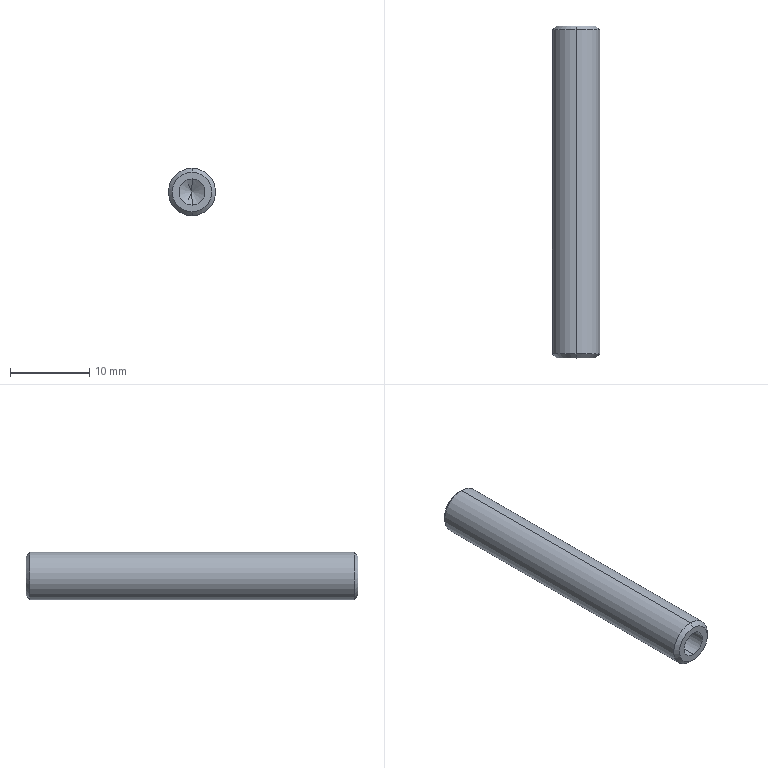Part | STEP file | 0-09-18 Guide shaft D6X50 | 1 solid | 16 faces | box 6 x 42 x 6 mm | volume 1005 mm3 | cone 8 | cylinder 6 | plane 2 | commonest cylinder face diameters 3.3 x4 6 x2
STEP:
#1=CARTESIAN_POINT('',(0.,0.,0.));
#2=DIRECTION('',(0.,0.,1.));
#3=DIRECTION('',(1.,0.,0.));
#4=AXIS2_PLACEMENT_3D('',#1,#2,#3);
#5=CARTESIAN_POINT('',(0.,10.1,-1.65));
#6=VERTEX_POINT('',#5);
#7=CARTESIAN_POINT('',(0.,0.,-1.65));
#8=VERTEX_POINT('',#7);
#9=CARTESIAN_POINT('',(0.,0.,-1.65));
#10=DIRECTION('',(0.,-1.,0.));
#11=VECTOR('',#10,1.);
#12=LINE('',#9,#11);
#13=CARTESIAN_POINT('',(0.,0.,0.));
#14=DIRECTION('',(0.,-1.,0.));
#15=DIRECTION('',(0.,0.,-1.));
#16=AXIS2_PLACEMENT_3D('',#13,#14,#15);
#17=CYLINDRICAL_SURFACE('',#16,1.65);
#18=CARTESIAN_POINT('',(6.283,0.));
#19=DIRECTION('',(0.,1.));
#20=VECTOR('',#19,1.);
#21=LINE('',#18,#20);
#22=(GEOMETRIC_REPRESENTATION_CONTEXT(2)PARAMETRIC_REPRESENTATION_CONTEXT()REPRESENTATION_CONTEXT('',''));
#23=DEFINITIONAL_REPRESENTATION('',(#21),#22);
#24=PCURVE('',#17,#23);
#25=CARTESIAN_POINT('',(0.,0.,0.));
#26=DIRECTION('',(0.,-1.,0.));
#27=DIRECTION('',(0.,0.,-1.));
#28=AXIS2_PLACEMENT_3D('',#25,#26,#27);
#29=CYLINDRICAL_SURFACE('',#28,1.65);
#30=CARTESIAN_POINT('',(0.,0.));
#31=DIRECTION('',(0.,1.));
#32=VECTOR('',#31,1.);
#33=LINE('',#30,#32);
#34=(GEOMETRIC_REPRESENTATION_CONTEXT(2)PARAMETRIC_REPRESENTATION_CONTEXT()REPRESENTATION_CONTEXT('',''));
#35=DEFINITIONAL_REPRESENTATION('',(#33),#34);
#36=PCURVE('',#29,#35);
#37=SURFACE_CURVE('',#12,(#24,#36),.PCURVE_S1.);
#38=EDGE_CURVE('',#6,#8,#37,.T.);
#39=ORIENTED_EDGE('',*,*,#38,.T.);
#40=CARTESIAN_POINT('',(0.,0.,1.65));
#41=VERTEX_POINT('',#40);
#42=CARTESIAN_POINT('',(0.,0.,0.));
#43=DIRECTION('',(0.,-1.,0.));
#44=DIRECTION('',(0.,0.,-1.));
#45=AXIS2_PLACEMENT_3D('',#42,#43,#44);
#46=CIRCLE('',#45,1.65);
#47=CARTESIAN_POINT('',(0.,0.));
#48=DIRECTION('',(1.,0.));
#49=VECTOR('',#48,1.);
#50=LINE('',#47,#49);
#51=(GEOMETRIC_REPRESENTATION_CONTEXT(2)PARAMETRIC_REPRESENTATION_CONTEXT()REPRESENTATION_CONTEXT('',''));
#52=DEFINITIONAL_REPRESENTATION('',(#50),#51);
#53=PCURVE('',#17,#52);
#54=CARTESIAN_POINT('',(0.,0.,0.));
#55=DIRECTION('',(0.,1.,0.));
#56=DIRECTION('',(0.,0.,1.));
#57=AXIS2_PLACEMENT_3D('',#54,#55,#56);
#58=PLANE('',#57);
#59=CARTESIAN_POINT('',(-1.65,0.));
#60=CARTESIAN_POINT('',(-1.65,2.858));
#61=CARTESIAN_POINT('',(0.825,1.429));
#62=CARTESIAN_POINT('',(3.3,0.));
#63=CARTESIAN_POINT('',(0.825,-1.429));
#64=CARTESIAN_POINT('',(-1.65,-2.858));
#65=CARTESIAN_POINT('',(-1.65,0.));
#66=(BOUNDED_CURVE()B_SPLINE_CURVE(2,(#59,#60,#61,#62,#63,#64,#65),.UNSPECIFIED.,.T.,.F.)B_SPLINE_CURVE_WITH_KNOTS((1,2,2,2,2,1),(-2.094,0.,2.094,4.189,6.283,8.378),.UNSPECIFIED.)CURVE()GEOMETRIC_REPRESENTATION_ITEM()RATIONAL_B_SPLINE_CURVE((1.,0.5,1.,0.5,1.,0.5,1.))REPRESENTATION_ITEM(''));
#67=(GEOMETRIC_REPRESENTATION_CONTEXT(2)PARAMETRIC_REPRESENTATION_CONTEXT()REPRESENTATION_CONTEXT('',''));
#68=DEFINITIONAL_REPRESENTATION('',(#66),#67);
#69=PCURVE('',#58,#68);
#70=SURFACE_CURVE('',#46,(#53,#69),.PCURVE_S1.);
#71=EDGE_CURVE('',#41,#8,#70,.T.);
#72=ORIENTED_EDGE('',*,*,#71,.F.);
#73=CARTESIAN_POINT('',(0.,10.1,1.65));
#74=VERTEX_POINT('',#73);
#75=CARTESIAN_POINT('',(0.,0.,1.65));
#76=DIRECTION('',(0.,-1.,0.));
#77=VECTOR('',#76,1.);
#78=LINE('',#75,#77);
#79=CARTESIAN_POINT('',(3.142,0.));
#80=DIRECTION('',(0.,1.));
#81=VECTOR('',#80,1.);
#82=LINE('',#79,#81);
#83=(GEOMETRIC_REPRESENTATION_CONTEXT(2)PARAMETRIC_REPRESENTATION_CONTEXT()REPRESENTATION_CONTEXT('',''));
#84=DEFINITIONAL_REPRESENTATION('',(#82),#83);
#85=PCURVE('',#17,#84);
#86=CARTESIAN_POINT('',(3.142,0.));
#87=DIRECTION('',(0.,1.));
#88=VECTOR('',#87,1.);
#89=LINE('',#86,#88);
#90=(GEOMETRIC_REPRESENTATION_CONTEXT(2)PARAMETRIC_REPRESENTATION_CONTEXT()REPRESENTATION_CONTEXT('',''));
#91=DEFINITIONAL_REPRESENTATION('',(#89),#90);
#92=PCURVE('',#29,#91);
#93=SURFACE_CURVE('',#78,(#85,#92),.PCURVE_S1.);
#94=EDGE_CURVE('',#74,#41,#93,.T.);
#95=ORIENTED_EDGE('',*,*,#94,.F.);
#96=CARTESIAN_POINT('',(0.,10.1,0.));
#97=DIRECTION('',(0.,-1.,0.));
#98=DIRECTION('',(0.,0.,-1.));
#99=AXIS2_PLACEMENT_3D('',#96,#97,#98);
#100=CIRCLE('',#99,1.65);
#101=CARTESIAN_POINT('',(0.,-10.1));
#102=DIRECTION('',(1.,0.));
#103=VECTOR('',#102,1.);
#104=LINE('',#101,#103);
#105=(GEOMETRIC_REPRESENTATION_CONTEXT(2)PARAMETRIC_REPRESENTATION_CONTEXT()REPRESENTATION_CONTEXT('',''));
#106=DEFINITIONAL_REPRESENTATION('',(#104),#105);
#107=PCURVE('',#17,#106);
#108=CARTESIAN_POINT('',(0.,10.1,0.));
#109=DIRECTION('',(0.,-1.,0.));
#110=DIRECTION('',(0.,0.,-1.));
#111=AXIS2_PLACEMENT_3D('',#108,#109,#110);
#112=CONICAL_SURFACE('',#111,1.65,1.03);
#113=CARTESIAN_POINT('',(0.,0.));
#114=DIRECTION('',(1.,0.));
#115=VECTOR('',#114,1.);
#116=LINE('',#113,#115);
#117=(GEOMETRIC_REPRESENTATION_CONTEXT(2)PARAMETRIC_REPRESENTATION_CONTEXT()REPRESENTATION_CONTEXT('',''));
#118=DEFINITIONAL_REPRESENTATION('',(#116),#117);
#119=PCURVE('',#112,#118);
#120=SURFACE_CURVE('',#100,(#107,#119),.PCURVE_S1.);
#121=EDGE_CURVE('',#74,#6,#120,.T.);
#122=ORIENTED_EDGE('',*,*,#121,.T.);
#123=EDGE_LOOP('',(#39,#72,#95,#122));
#124=FACE_BOUND('',#123,.F.);
#125=ADVANCED_FACE('',(#124),#17,.F.);
#126=ORIENTED_EDGE('',*,*,#121,.F.);
#127=CARTESIAN_POINT('',(0.,11.091,0.));
#128=VERTEX_POINT('',#127);
#129=CARTESIAN_POINT('',(0.,10.1,1.65));
#130=DIRECTION('',(0.,-0.515,0.8572));
#131=VECTOR('',#130,1.);
#132=LINE('',#129,#131);
#133=CARTESIAN_POINT('',(3.142,0.));
#134=DIRECTION('',(0.,1.));
#135=VECTOR('',#134,1.);
#136=LINE('',#133,#135);
#137=(GEOMETRIC_REPRESENTATION_CONTEXT(2)PARAMETRIC_REPRESENTATION_CONTEXT()REPRESENTATION_CONTEXT('',''));
#138=DEFINITIONAL_REPRESENTATION('',(#136),#137);
#139=PCURVE('',#112,#138);
#140=CARTESIAN_POINT('',(0.,10.1,0.));
#141=DIRECTION('',(0.,-1.,0.));
#142=DIRECTION('',(0.,0.,-1.));
#143=AXIS2_PLACEMENT_3D('',#140,#141,#142);
#144=CONICAL_SURFACE('',#143,1.65,1.03);
#145=CARTESIAN_POINT('',(3.142,0.));
#146=DIRECTION('',(0.,1.));
#147=VECTOR('',#146,1.);
#148=LINE('',#145,#147);
#149=(GEOMETRIC_REPRESENTATION_CONTEXT(2)PARAMETRIC_REPRESENTATION_CONTEXT()REPRESENTATION_CONTEXT('',''));
#150=DEFINITIONAL_REPRESENTATION('',(#148),#149);
#151=PCURVE('',#144,#150);
#152=SURFACE_CURVE('',#132,(#139,#151),.PCURVE_S1.);
#153=EDGE_CURVE('',#128,#74,#152,.T.);
#154=ORIENTED_EDGE('',*,*,#153,.F.);
#155=CARTESIAN_POINT('',(0.,10.1,-1.65));
#156=DIRECTION('',(0.,-0.515,-0.8572));
#157=VECTOR('',#156,1.);
#158=LINE('',#155,#157);
#159=CARTESIAN_POINT('',(6.283,0.));
#160=DIRECTION('',(0.,1.));
#161=VECTOR('',#160,1.);
#162=LINE('',#159,#161);
#163=(GEOMETRIC_REPRESENTATION_CONTEXT(2)PARAMETRIC_REPRESENTATION_CONTEXT()REPRESENTATION_CONTEXT('',''));
#164=DEFINITIONAL_REPRESENTATION('',(#162),#163);
#165=PCURVE('',#112,#164);
#166=CARTESIAN_POINT('',(0.,0.));
#167=DIRECTION('',(0.,1.));
#168=VECTOR('',#167,1.);
#169=LINE('',#166,#168);
#170=(GEOMETRIC_REPRESENTATION_CONTEXT(2)PARAMETRIC_REPRESENTATION_CONTEXT()REPRESENTATION_CONTEXT('',''));
#171=DEFINITIONAL_REPRESENTATION('',(#169),#170);
#172=PCURVE('',#144,#171);
#173=SURFACE_CURVE('',#158,(#165,#172),.PCURVE_S1.);
#174=EDGE_CURVE('',#128,#6,#173,.T.);
#175=ORIENTED_EDGE('',*,*,#174,.T.);
#176=EDGE_LOOP('',(#126,#154,#175));
#177=FACE_BOUND('',#176,.F.);
#178=ADVANCED_FACE('',(#177),#112,.F.);
#179=CARTESIAN_POINT('',(0.,31.9,1.65));
#180=VERTEX_POINT('',#179);
#181=CARTESIAN_POINT('',(0.,42.,1.65));
#182=VERTEX_POINT('',#181);
#183=CARTESIAN_POINT('',(0.,42.,1.65));
#184=DIRECTION('',(0.,1.,0.));
#185=VECTOR('',#184,1.);
#186=LINE('',#183,#185);
#187=CARTESIAN_POINT('',(0.,42.,0.));
#188=DIRECTION('',(0.,1.,0.));
#189=DIRECTION('',(0.,0.,1.));
#190=AXIS2_PLACEMENT_3D('',#187,#188,#189);
#191=CYLINDRICAL_SURFACE('',#190,1.65);
#192=CARTESIAN_POINT('',(6.283,0.));
#193=DIRECTION('',(0.,1.));
#194=VECTOR('',#193,1.);
#195=LINE('',#192,#194);
#196=(GEOMETRIC_REPRESENTATION_CONTEXT(2)PARAMETRIC_REPRESENTATION_CONTEXT()REPRESENTATION_CONTEXT('',''));
#197=DEFINITIONAL_REPRESENTATION('',(#195),#196);
#198=PCURVE('',#191,#197);
#199=CARTESIAN_POINT('',(0.,42.,0.));
#200=DIRECTION('',(0.,1.,0.));
#201=DIRECTION('',(0.,0.,1.));
#202=AXIS2_PLACEMENT_3D('',#199,#200,#201);
#203=CYLINDRICAL_SURFACE('',#202,1.65);
#204=CARTESIAN_POINT('',(0.,0.));
#205=DIRECTION('',(0.,1.));
#206=VECTOR('',#205,1.);
#207=LINE('',#204,#206);
#208=(GEOMETRIC_REPRESENTATION_CONTEXT(2)PARAMETRIC_REPRESENTATION_CONTEXT()REPRESENTATION_CONTEXT('',''));
#209=DEFINITIONAL_REPRESENTATION('',(#207),#208);
#210=PCURVE('',#203,#209);
#211=SURFACE_CURVE('',#186,(#198,#210),.PCURVE_S1.);
#212=EDGE_CURVE('',#180,#182,#211,.T.);
#213=ORIENTED_EDGE('',*,*,#212,.T.);
#214=CARTESIAN_POINT('',(0.,42.,-1.65));
#215=VERTEX_POINT('',#214);
#216=CARTESIAN_POINT('',(0.,42.,0.));
#217=DIRECTION('',(0.,1.,0.));
#218=DIRECTION('',(0.,0.,1.));
#219=AXIS2_PLACEMENT_3D('',#216,#217,#218);
#220=CIRCLE('',#219,1.65);
#221=CARTESIAN_POINT('',(0.,0.));
#222=DIRECTION('',(1.,0.));
#223=VECTOR('',#222,1.);
#224=LINE('',#221,#223);
#225=(GEOMETRIC_REPRESENTATION_CONTEXT(2)PARAMETRIC_REPRESENTATION_CONTEXT()REPRESENTATION_CONTEXT('',''));
#226=DEFINITIONAL_REPRESENTATION('',(#224),#225);
#227=PCURVE('',#191,#226);
#228=CARTESIAN_POINT('',(0.,42.,0.));
#229=DIRECTION('',(0.,-1.,0.));
#230=DIRECTION('',(0.,0.,-1.));
#231=AXIS2_PLACEMENT_3D('',#228,#229,#230);
#232=PLANE('',#231);
#233=CARTESIAN_POINT('',(-1.65,0.));
#234=CARTESIAN_POINT('',(-1.65,2.858));
#235=CARTESIAN_POINT('',(0.825,1.429));
#236=CARTESIAN_POINT('',(3.3,0.));
#237=CARTESIAN_POINT('',(0.825,-1.429));
#238=CARTESIAN_POINT('',(-1.65,-2.858));
#239=CARTESIAN_POINT('',(-1.65,0.));
#240=(BOUNDED_CURVE()B_SPLINE_CURVE(2,(#233,#234,#235,#236,#237,#238,#239),.UNSPECIFIED.,.T.,.F.)B_SPLINE_CURVE_WITH_KNOTS((1,2,2,2,2,1),(-2.094,0.,2.094,4.189,6.283,8.378),.UNSPECIFIED.)CURVE()GEOMETRIC_REPRESENTATION_ITEM()RATIONAL_B_SPLINE_CURVE((1.,0.5,1.,0.5,1.,0.5,1.))REPRESENTATION_ITEM(''));
#241=(GEOMETRIC_REPRESENTATION_CONTEXT(2)PARAMETRIC_REPRESENTATION_CONTEXT()REPRESENTATION_CONTEXT('',''));
#242=DEFINITIONAL_REPRESENTATION('',(#240),#241);
#243=PCURVE('',#232,#242);
#244=SURFACE_CURVE('',#220,(#227,#243),.PCURVE_S1.);
#245=EDGE_CURVE('',#215,#182,#244,.T.);
#246=ORIENTED_EDGE('',*,*,#245,.F.);
#247=CARTESIAN_POINT('',(0.,31.9,-1.65));
#248=VERTEX_POINT('',#247);
#249=CARTESIAN_POINT('',(0.,42.,-1.65));
#250=DIRECTION('',(0.,1.,0.));
#251=VECTOR('',#250,1.);
#252=LINE('',#249,#251);
#253=CARTESIAN_POINT('',(3.142,0.));
#254=DIRECTION('',(0.,1.));
#255=VECTOR('',#254,1.);
#256=LINE('',#253,#255);
#257=(GEOMETRIC_REPRESENTATION_CONTEXT(2)PARAMETRIC_REPRESENTATION_CONTEXT()REPRESENTATION_CONTEXT('',''));
#258=DEFINITIONAL_REPRESENTATION('',(#256),#257);
#259=PCURVE('',#191,#258);
#260=CARTESIAN_POINT('',(3.142,0.));
#261=DIRECTION('',(0.,1.));
#262=VECTOR('',#261,1.);
#263=LINE('',#260,#262);
#264=(GEOMETRIC_REPRESENTATION_CONTEXT(2)PARAMETRIC_REPRESENTATION_CONTEXT()REPRESENTATION_CONTEXT('',''));
#265=DEFINITIONAL_REPRESENTATION('',(#263),#264);
#266=PCURVE('',#203,#265);
#267=SURFACE_CURVE('',#252,(#259,#266),.PCURVE_S1.);
#268=EDGE_CURVE('',#248,#215,#267,.T.);
#269=ORIENTED_EDGE('',*,*,#268,.F.);
#270=CARTESIAN_POINT('',(0.,31.9,0.));
#271=DIRECTION('',(0.,1.,0.));
#272=DIRECTION('',(0.,0.,1.));
#273=AXIS2_PLACEMENT_3D('',#270,#271,#272);
#274=CIRCLE('',#273,1.65);
#275=CARTESIAN_POINT('',(0.,-10.1));
#276=DIRECTION('',(1.,0.));
#277=VECTOR('',#276,1.);
#278=LINE('',#275,#277);
#279=(GEOMETRIC_REPRESENTATION_CONTEXT(2)PARAMETRIC_REPRESENTATION_CONTEXT()REPRESENTATION_CONTEXT('',''));
#280=DEFINITIONAL_REPRESENTATION('',(#278),#279);
#281=PCURVE('',#191,#280);
#282=CARTESIAN_POINT('',(0.,31.9,0.));
#283=DIRECTION('',(0.,1.,0.));
#284=DIRECTION('',(0.,0.,1.));
#285=AXIS2_PLACEMENT_3D('',#282,#283,#284);
#286=CONICAL_SURFACE('',#285,1.65,1.03);
#287=CARTESIAN_POINT('',(0.,0.));
#288=DIRECTION('',(1.,0.));
#289=VECTOR('',#288,1.);
#290=LINE('',#287,#289);
#291=(GEOMETRIC_REPRESENTATION_CONTEXT(2)PARAMETRIC_REPRESENTATION_CONTEXT()REPRESENTATION_CONTEXT('',''));
#292=DEFINITIONAL_REPRESENTATION('',(#290),#291);
#293=PCURVE('',#286,#292);
#294=SURFACE_CURVE('',#274,(#281,#293),.PCURVE_S1.);
#295=EDGE_CURVE('',#248,#180,#294,.T.);
#296=ORIENTED_EDGE('',*,*,#295,.T.);
#297=EDGE_LOOP('',(#213,#246,#269,#296));
#298=FACE_BOUND('',#297,.F.);
#299=ADVANCED_FACE('',(#298),#191,.F.);
#300=ORIENTED_EDGE('',*,*,#295,.F.);
#301=CARTESIAN_POINT('',(0.,30.909,0.));
#302=VERTEX_POINT('',#301);
#303=CARTESIAN_POINT('',(0.,31.9,-1.65));
#304=DIRECTION('',(0.,0.515,-0.8572));
#305=VECTOR('',#304,1.);
#306=LINE('',#303,#305);
#307=CARTESIAN_POINT('',(3.142,0.));
#308=DIRECTION('',(0.,1.));
#309=VECTOR('',#308,1.);
#310=LINE('',#307,#309);
#311=(GEOMETRIC_REPRESENTATION_CONTEXT(2)PARAMETRIC_REPRESENTATION_CONTEXT()REPRESENTATION_CONTEXT('',''));
#312=DEFINITIONAL_REPRESENTATION('',(#310),#311);
#313=PCURVE('',#286,#312);
#314=CARTESIAN_POINT('',(0.,31.9,0.));
#315=DIRECTION('',(0.,1.,0.));
#316=DIRECTION('',(0.,0.,1.));
#317=AXIS2_PLACEMENT_3D('',#314,#315,#316);
#318=CONICAL_SURFACE('',#317,1.65,1.03);
#319=CARTESIAN_POINT('',(3.142,0.));
#320=DIRECTION('',(0.,1.));
#321=VECTOR('',#320,1.);
#322=LINE('',#319,#321);
#323=(GEOMETRIC_REPRESENTATION_CONTEXT(2)PARAMETRIC_REPRESENTATION_CONTEXT()REPRESENTATION_CONTEXT('',''));
#324=DEFINITIONAL_REPRESENTATION('',(#322),#323);
#325=PCURVE('',#318,#324);
#326=SURFACE_CURVE('',#306,(#313,#325),.PCURVE_S1.);
#327=EDGE_CURVE('',#302,#248,#326,.T.);
#328=ORIENTED_EDGE('',*,*,#327,.F.);
#329=CARTESIAN_POINT('',(0.,31.9,1.65));
#330=DIRECTION('',(0.,0.515,0.8572));
#331=VECTOR('',#330,1.);
#332=LINE('',#329,#331);
#333=CARTESIAN_POINT('',(6.283,0.));
#334=DIRECTION('',(0.,1.));
#335=VECTOR('',#334,1.);
#336=LINE('',#333,#335);
#337=(GEOMETRIC_REPRESENTATION_CONTEXT(2)PARAMETRIC_REPRESENTATION_CONTEXT()REPRESENTATION_CONTEXT('',''));
#338=DEFINITIONAL_REPRESENTATION('',(#336),#337);
#339=PCURVE('',#286,#338);
#340=CARTESIAN_POINT('',(0.,0.));
#341=DIRECTION('',(0.,1.));
#342=VECTOR('',#341,1.);
#343=LINE('',#340,#342);
#344=(GEOMETRIC_REPRESENTATION_CONTEXT(2)PARAMETRIC_REPRESENTATION_CONTEXT()REPRESENTATION_CONTEXT('',''));
#345=DEFINITIONAL_REPRESENTATION('',(#343),#344);
#346=PCURVE('',#318,#345);
#347=SURFACE_CURVE('',#332,(#339,#346),.PCURVE_S1.);
#348=EDGE_CURVE('',#302,#180,#347,.T.);
#349=ORIENTED_EDGE('',*,*,#348,.T.);
#350=EDGE_LOOP('',(#300,#328,#349));
#351=FACE_BOUND('',#350,.F.);
#352=ADVANCED_FACE('',(#351),#286,.F.);
#353=CARTESIAN_POINT('',(0.,42.,2.5));
#354=VERTEX_POINT('',#353);
#355=CARTESIAN_POINT('',(0.,42.,-2.5));
#356=VERTEX_POINT('',#355);
#357=CARTESIAN_POINT('',(0.,42.,0.));
#358=DIRECTION('',(0.,1.,0.));
#359=DIRECTION('',(0.,0.,-1.));
#360=AXIS2_PLACEMENT_3D('',#357,#358,#359);
#361=CIRCLE('',#360,2.5);
#362=CARTESIAN_POINT('',(0.,41.5,0.));
#363=DIRECTION('',(0.,-1.,0.));
#364=DIRECTION('',(0.,0.,-1.));
#365=AXIS2_PLACEMENT_3D('',#362,#363,#364);
#366=CONICAL_SURFACE('',#365,3.,0.7854);
#367=CARTESIAN_POINT('',(6.283,-0.5));
#368=DIRECTION('',(-1.,0.));
#369=VECTOR('',#368,1.);
#370=LINE('',#367,#369);
#371=(GEOMETRIC_REPRESENTATION_CONTEXT(2)PARAMETRIC_REPRESENTATION_CONTEXT()REPRESENTATION_CONTEXT('',''));
#372=DEFINITIONAL_REPRESENTATION('',(#370),#371);
#373=PCURVE('',#366,#372);
#374=CARTESIAN_POINT('',(2.5,0.));
#375=CARTESIAN_POINT('',(2.5,-4.33));
#376=CARTESIAN_POINT('',(-1.25,-2.165));
#377=CARTESIAN_POINT('',(-5.,0.));
#378=CARTESIAN_POINT('',(-1.25,2.165));
#379=CARTESIAN_POINT('',(2.5,4.33));
#380=CARTESIAN_POINT('',(2.5,0.));
#381=(BOUNDED_CURVE()B_SPLINE_CURVE(2,(#374,#375,#376,#377,#378,#379,#380),.UNSPECIFIED.,.T.,.F.)B_SPLINE_CURVE_WITH_KNOTS((1,2,2,2,2,1),(-2.094,0.,2.094,4.189,6.283,8.378),.UNSPECIFIED.)CURVE()GEOMETRIC_REPRESENTATION_ITEM()RATIONAL_B_SPLINE_CURVE((1.,0.5,1.,0.5,1.,0.5,1.))REPRESENTATION_ITEM(''));
#382=(GEOMETRIC_REPRESENTATION_CONTEXT(2)PARAMETRIC_REPRESENTATION_CONTEXT()REPRESENTATION_CONTEXT('',''));
#383=DEFINITIONAL_REPRESENTATION('',(#381),#382);
#384=PCURVE('',#232,#383);
#385=SURFACE_CURVE('',#361,(#373,#384),.PCURVE_S1.);
#386=EDGE_CURVE('',#354,#356,#385,.T.);
#387=ORIENTED_EDGE('',*,*,#386,.F.);
#388=CARTESIAN_POINT('',(0.,41.5,3.));
#389=VERTEX_POINT('',#388);
#390=CARTESIAN_POINT('',(0.,41.5,3.));
#391=DIRECTION('',(0.,-0.7071,0.7071));
#392=VECTOR('',#391,1.);
#393=LINE('',#390,#392);
#394=CARTESIAN_POINT('',(3.142,0.));
#395=DIRECTION('',(0.,1.));
#396=VECTOR('',#395,1.);
#397=LINE('',#394,#396);
#398=(GEOMETRIC_REPRESENTATION_CONTEXT(2)PARAMETRIC_REPRESENTATION_CONTEXT()REPRESENTATION_CONTEXT('',''));
#399=DEFINITIONAL_REPRESENTATION('',(#397),#398);
#400=PCURVE('',#366,#399);
#401=CARTESIAN_POINT('',(0.,41.5,0.));
#402=DIRECTION('',(0.,-1.,0.));
#403=DIRECTION('',(0.,0.,-1.));
#404=AXIS2_PLACEMENT_3D('',#401,#402,#403);
#405=CONICAL_SURFACE('',#404,3.,0.7854);
#406=CARTESIAN_POINT('',(3.142,0.));
#407=DIRECTION('',(0.,1.));
#408=VECTOR('',#407,1.);
#409=LINE('',#406,#408);
#410=(GEOMETRIC_REPRESENTATION_CONTEXT(2)PARAMETRIC_REPRESENTATION_CONTEXT()REPRESENTATION_CONTEXT('',''));
#411=DEFINITIONAL_REPRESENTATION('',(#409),#410);
#412=PCURVE('',#405,#411);
#413=SURFACE_CURVE('',#393,(#400,#412),.PCURVE_S1.);
#414=EDGE_CURVE('',#354,#389,#413,.T.);
#415=ORIENTED_EDGE('',*,*,#414,.T.);
#416=CARTESIAN_POINT('',(0.,41.5,-3.));
#417=VERTEX_POINT('',#416);
#418=CARTESIAN_POINT('',(0.,41.5,0.));
#419=DIRECTION('',(0.,-1.,0.));
#420=DIRECTION('',(0.,0.,-1.));
#421=AXIS2_PLACEMENT_3D('',#418,#419,#420);
#422=CIRCLE('',#421,3.);
#423=CARTESIAN_POINT('',(0.,0.));
#424=DIRECTION('',(1.,0.));
#425=VECTOR('',#424,1.);
#426=LINE('',#423,#425);
#427=(GEOMETRIC_REPRESENTATION_CONTEXT(2)PARAMETRIC_REPRESENTATION_CONTEXT()REPRESENTATION_CONTEXT('',''));
#428=DEFINITIONAL_REPRESENTATION('',(#426),#427);
#429=PCURVE('',#366,#428);
#430=CARTESIAN_POINT('',(0.,0.,0.));
#431=DIRECTION('',(0.,-1.,0.));
#432=DIRECTION('',(0.,0.,-1.));
#433=AXIS2_PLACEMENT_3D('',#430,#431,#432);
#434=CYLINDRICAL_SURFACE('',#433,3.);
#435=CARTESIAN_POINT('',(0.,-41.5));
#436=DIRECTION('',(1.,0.));
#437=VECTOR('',#436,1.);
#438=LINE('',#435,#437);
#439=(GEOMETRIC_REPRESENTATION_CONTEXT(2)PARAMETRIC_REPRESENTATION_CONTEXT()REPRESENTATION_CONTEXT('',''));
#440=DEFINITIONAL_REPRESENTATION('',(#438),#439);
#441=PCURVE('',#434,#440);
#442=SURFACE_CURVE('',#422,(#429,#441),.PCURVE_S1.);
#443=EDGE_CURVE('',#417,#389,#442,.T.);
#444=ORIENTED_EDGE('',*,*,#443,.F.);
#445=CARTESIAN_POINT('',(0.,41.5,-3.));
#446=DIRECTION('',(0.,-0.7071,-0.7071));
#447=VECTOR('',#446,1.);
#448=LINE('',#445,#447);
#449=CARTESIAN_POINT('',(0.,0.));
#450=DIRECTION('',(0.,1.));
#451=VECTOR('',#450,1.);
#452=LINE('',#449,#451);
#453=(GEOMETRIC_REPRESENTATION_CONTEXT(2)PARAMETRIC_REPRESENTATION_CONTEXT()REPRESENTATION_CONTEXT('',''));
#454=DEFINITIONAL_REPRESENTATION('',(#452),#453);
#455=PCURVE('',#366,#454);
#456=CARTESIAN_POINT('',(6.283,0.));
#457=DIRECTION('',(0.,1.));
#458=VECTOR('',#457,1.);
#459=LINE('',#456,#458);
#460=(GEOMETRIC_REPRESENTATION_CONTEXT(2)PARAMETRIC_REPRESENTATION_CONTEXT()REPRESENTATION_CONTEXT('',''));
#461=DEFINITIONAL_REPRESENTATION('',(#459),#460);
#462=PCURVE('',#405,#461);
#463=SURFACE_CURVE('',#448,(#455,#462),.PCURVE_S1.);
#464=EDGE_CURVE('',#356,#417,#463,.T.);
#465=ORIENTED_EDGE('',*,*,#464,.F.);
#466=EDGE_LOOP('',(#387,#415,#444,#465));
#467=FACE_BOUND('',#466,.T.);
#468=ADVANCED_FACE('',(#467),#366,.T.);
#469=CARTESIAN_POINT('',(0.,0.,-2.5));
#470=VERTEX_POINT('',#469);
#471=CARTESIAN_POINT('',(0.,0.,2.5));
#472=VERTEX_POINT('',#471);
#473=CARTESIAN_POINT('',(0.,0.,0.));
#474=DIRECTION('',(0.,-1.,0.));
#475=DIRECTION('',(0.,0.,1.));
#476=AXIS2_PLACEMENT_3D('',#473,#474,#475);
#477=CIRCLE('',#476,2.5);
#478=CARTESIAN_POINT('',(0.,0.,0.));
#479=DIRECTION('',(0.,1.,0.));
#480=DIRECTION('',(0.,0.,1.));
#481=AXIS2_PLACEMENT_3D('',#478,#479,#480);
#482=CONICAL_SURFACE('',#481,2.5,0.7854);
#483=CARTESIAN_POINT('',(6.283,0.));
#484=DIRECTION('',(-1.,0.));
#485=VECTOR('',#484,1.);
#486=LINE('',#483,#485);
#487=(GEOMETRIC_REPRESENTATION_CONTEXT(2)PARAMETRIC_REPRESENTATION_CONTEXT()REPRESENTATION_CONTEXT('',''));
#488=DEFINITIONAL_REPRESENTATION('',(#486),#487);
#489=PCURVE('',#482,#488);
#490=CARTESIAN_POINT('',(2.5,0.));
#491=CARTESIAN_POINT('',(2.5,-4.33));
#492=CARTESIAN_POINT('',(-1.25,-2.165));
#493=CARTESIAN_POINT('',(-5.,0.));
#494=CARTESIAN_POINT('',(-1.25,2.165));
#495=CARTESIAN_POINT('',(2.5,4.33));
#496=CARTESIAN_POINT('',(2.5,0.));
#497=(BOUNDED_CURVE()B_SPLINE_CURVE(2,(#490,#491,#492,#493,#494,#495,#496),.UNSPECIFIED.,.T.,.F.)B_SPLINE_CURVE_WITH_KNOTS((1,2,2,2,2,1),(-2.094,0.,2.094,4.189,6.283,8.378),.UNSPECIFIED.)CURVE()GEOMETRIC_REPRESENTATION_ITEM()RATIONAL_B_SPLINE_CURVE((1.,0.5,1.,0.5,1.,0.5,1.))REPRESENTATION_ITEM(''));
#498=(GEOMETRIC_REPRESENTATION_CONTEXT(2)PARAMETRIC_REPRESENTATION_CONTEXT()REPRESENTATION_CONTEXT('',''));
#499=DEFINITIONAL_REPRESENTATION('',(#497),#498);
#500=PCURVE('',#58,#499);
#501=SURFACE_CURVE('',#477,(#489,#500),.PCURVE_S1.);
#502=EDGE_CURVE('',#470,#472,#501,.T.);
#503=ORIENTED_EDGE('',*,*,#502,.F.);
#504=CARTESIAN_POINT('',(0.,0.5,-3.));
#505=VERTEX_POINT('',#504);
#506=CARTESIAN_POINT('',(0.,0.,-2.5));
#507=DIRECTION('',(0.,0.7071,-0.7071));
#508=VECTOR('',#507,1.);
#509=LINE('',#506,#508);
#510=CARTESIAN_POINT('',(3.142,0.));
#511=DIRECTION('',(0.,1.));
#512=VECTOR('',#511,1.);
#513=LINE('',#510,#512);
#514=(GEOMETRIC_REPRESENTATION_CONTEXT(2)PARAMETRIC_REPRESENTATION_CONTEXT()REPRESENTATION_CONTEXT('',''));
#515=DEFINITIONAL_REPRESENTATION('',(#513),#514);
#516=PCURVE('',#482,#515);
#517=CARTESIAN_POINT('',(0.,0.,0.));
#518=DIRECTION('',(0.,1.,0.));
#519=DIRECTION('',(0.,0.,1.));
#520=AXIS2_PLACEMENT_3D('',#517,#518,#519);
#521=CONICAL_SURFACE('',#520,2.5,0.7854);
#522=CARTESIAN_POINT('',(3.142,0.));
#523=DIRECTION('',(0.,1.));
#524=VECTOR('',#523,1.);
#525=LINE('',#522,#524);
#526=(GEOMETRIC_REPRESENTATION_CONTEXT(2)PARAMETRIC_REPRESENTATION_CONTEXT()REPRESENTATION_CONTEXT('',''));
#527=DEFINITIONAL_REPRESENTATION('',(#525),#526);
#528=PCURVE('',#521,#527);
#529=SURFACE_CURVE('',#509,(#516,#528),.PCURVE_S1.);
#530=EDGE_CURVE('',#470,#505,#529,.T.);
#531=ORIENTED_EDGE('',*,*,#530,.T.);
#532=CARTESIAN_POINT('',(0.,0.5,3.));
#533=VERTEX_POINT('',#532);
#534=CARTESIAN_POINT('',(0.,0.5,0.));
#535=DIRECTION('',(0.,1.,0.));
#536=DIRECTION('',(0.,0.,1.));
#537=AXIS2_PLACEMENT_3D('',#534,#535,#536);
#538=CIRCLE('',#537,3.);
#539=CARTESIAN_POINT('',(0.,0.5));
#540=DIRECTION('',(1.,0.));
#541=VECTOR('',#540,1.);
#542=LINE('',#539,#541);
#543=(GEOMETRIC_REPRESENTATION_CONTEXT(2)PARAMETRIC_REPRESENTATION_CONTEXT()REPRESENTATION_CONTEXT('',''));
#544=DEFINITIONAL_REPRESENTATION('',(#542),#543);
#545=PCURVE('',#482,#544);
#546=CARTESIAN_POINT('',(3.142,-0.5));
#547=DIRECTION('',(-1.,0.));
#548=VECTOR('',#547,1.);
#549=LINE('',#546,#548);
#550=(GEOMETRIC_REPRESENTATION_CONTEXT(2)PARAMETRIC_REPRESENTATION_CONTEXT()REPRESENTATION_CONTEXT('',''));
#551=DEFINITIONAL_REPRESENTATION('',(#549),#550);
#552=PCURVE('',#434,#551);
#553=SURFACE_CURVE('',#538,(#545,#552),.PCURVE_S1.);
#554=EDGE_CURVE('',#533,#505,#553,.T.);
#555=ORIENTED_EDGE('',*,*,#554,.F.);
#556=CARTESIAN_POINT('',(0.,0.,2.5));
#557=DIRECTION('',(0.,0.7071,0.7071));
#558=VECTOR('',#557,1.);
#559=LINE('',#556,#558);
#560=CARTESIAN_POINT('',(0.,0.));
#561=DIRECTION('',(0.,1.));
#562=VECTOR('',#561,1.);
#563=LINE('',#560,#562);
#564=(GEOMETRIC_REPRESENTATION_CONTEXT(2)PARAMETRIC_REPRESENTATION_CONTEXT()REPRESENTATION_CONTEXT('',''));
#565=DEFINITIONAL_REPRESENTATION('',(#563),#564);
#566=PCURVE('',#482,#565);
#567=CARTESIAN_POINT('',(6.283,0.));
#568=DIRECTION('',(0.,1.));
#569=VECTOR('',#568,1.);
#570=LINE('',#567,#569);
#571=(GEOMETRIC_REPRESENTATION_CONTEXT(2)PARAMETRIC_REPRESENTATION_CONTEXT()REPRESENTATION_CONTEXT('',''));
#572=DEFINITIONAL_REPRESENTATION('',(#570),#571);
#573=PCURVE('',#521,#572);
#574=SURFACE_CURVE('',#559,(#566,#573),.PCURVE_S1.);
#575=EDGE_CURVE('',#472,#533,#574,.T.);
#576=ORIENTED_EDGE('',*,*,#575,.F.);
#577=EDGE_LOOP('',(#503,#531,#555,#576));
#578=FACE_BOUND('',#577,.T.);
#579=ADVANCED_FACE('',(#578),#482,.T.);
#580=ORIENTED_EDGE('',*,*,#443,.T.);
#581=CARTESIAN_POINT('',(0.,0.,3.));
#582=DIRECTION('',(0.,-1.,0.));
#583=VECTOR('',#582,1.);
#584=LINE('',#581,#583);
#585=CARTESIAN_POINT('',(3.142,0.));
#586=DIRECTION('',(0.,1.));
#587=VECTOR('',#586,1.);
#588=LINE('',#585,#587);
#589=(GEOMETRIC_REPRESENTATION_CONTEXT(2)PARAMETRIC_REPRESENTATION_CONTEXT()REPRESENTATION_CONTEXT('',''));
#590=DEFINITIONAL_REPRESENTATION('',(#588),#589);
#591=PCURVE('',#434,#590);
#592=CARTESIAN_POINT('',(0.,0.,0.));
#593=DIRECTION('',(0.,-1.,0.));
#594=DIRECTION('',(0.,0.,-1.));
#595=AXIS2_PLACEMENT_3D('',#592,#593,#594);
#596=CYLINDRICAL_SURFACE('',#595,3.);
#597=CARTESIAN_POINT('',(3.142,0.));
#598=DIRECTION('',(0.,1.));
#599=VECTOR('',#598,1.);
#600=LINE('',#597,#599);
#601=(GEOMETRIC_REPRESENTATION_CONTEXT(2)PARAMETRIC_REPRESENTATION_CONTEXT()REPRESENTATION_CONTEXT('',''));
#602=DEFINITIONAL_REPRESENTATION('',(#600),#601);
#603=PCURVE('',#596,#602);
#604=SURFACE_CURVE('',#584,(#591,#603),.PCURVE_S1.);
#605=EDGE_CURVE('',#389,#533,#604,.T.);
#606=ORIENTED_EDGE('',*,*,#605,.T.);
#607=ORIENTED_EDGE('',*,*,#554,.T.);
#608=CARTESIAN_POINT('',(0.,0.,-3.));
#609=DIRECTION('',(0.,-1.,0.));
#610=VECTOR('',#609,1.);
#611=LINE('',#608,#610);
#612=CARTESIAN_POINT('',(0.,0.));
#613=DIRECTION('',(0.,1.));
#614=VECTOR('',#613,1.);
#615=LINE('',#612,#614);
#616=(GEOMETRIC_REPRESENTATION_CONTEXT(2)PARAMETRIC_REPRESENTATION_CONTEXT()REPRESENTATION_CONTEXT('',''));
#617=DEFINITIONAL_REPRESENTATION('',(#615),#616);
#618=PCURVE('',#434,#617);
#619=CARTESIAN_POINT('',(6.283,0.));
#620=DIRECTION('',(0.,1.));
#621=VECTOR('',#620,1.);
#622=LINE('',#619,#621);
#623=(GEOMETRIC_REPRESENTATION_CONTEXT(2)PARAMETRIC_REPRESENTATION_CONTEXT()REPRESENTATION_CONTEXT('',''));
#624=DEFINITIONAL_REPRESENTATION('',(#622),#623);
#625=PCURVE('',#596,#624);
#626=SURFACE_CURVE('',#611,(#618,#625),.PCURVE_S1.);
#627=EDGE_CURVE('',#417,#505,#626,.T.);
#628=ORIENTED_EDGE('',*,*,#627,.F.);
#629=EDGE_LOOP('',(#580,#606,#607,#628));
#630=FACE_BOUND('',#629,.T.);
#631=ADVANCED_FACE('',(#630),#434,.T.);
#632=CARTESIAN_POINT('',(0.,42.,0.));
#633=DIRECTION('',(0.,1.,0.));
#634=DIRECTION('',(0.,0.,1.));
#635=AXIS2_PLACEMENT_3D('',#632,#633,#634);
#636=CIRCLE('',#635,1.65);
#637=CARTESIAN_POINT('',(-1.65,0.));
#638=CARTESIAN_POINT('',(-1.65,2.858));
#639=CARTESIAN_POINT('',(0.825,1.429));
#640=CARTESIAN_POINT('',(3.3,0.));
#641=CARTESIAN_POINT('',(0.825,-1.429));
#642=CARTESIAN_POINT('',(-1.65,-2.858));
#643=CARTESIAN_POINT('',(-1.65,0.));
#644=(BOUNDED_CURVE()B_SPLINE_CURVE(2,(#637,#638,#639,#640,#641,#642,#643),.UNSPECIFIED.,.T.,.F.)B_SPLINE_CURVE_WITH_KNOTS((1,2,2,2,2,1),(-2.094,0.,2.094,4.189,6.283,8.378),.UNSPECIFIED.)CURVE()GEOMETRIC_REPRESENTATION_ITEM()RATIONAL_B_SPLINE_CURVE((1.,0.5,1.,0.5,1.,0.5,1.))REPRESENTATION_ITEM(''));
#645=(GEOMETRIC_REPRESENTATION_CONTEXT(2)PARAMETRIC_REPRESENTATION_CONTEXT()REPRESENTATION_CONTEXT('',''));
#646=DEFINITIONAL_REPRESENTATION('',(#644),#645);
#647=PCURVE('',#232,#646);
#648=CARTESIAN_POINT('',(0.,0.));
#649=DIRECTION('',(1.,0.));
#650=VECTOR('',#649,1.);
#651=LINE('',#648,#650);
#652=(GEOMETRIC_REPRESENTATION_CONTEXT(2)PARAMETRIC_REPRESENTATION_CONTEXT()REPRESENTATION_CONTEXT('',''));
#653=DEFINITIONAL_REPRESENTATION('',(#651),#652);
#654=PCURVE('',#203,#653);
#655=SURFACE_CURVE('',#636,(#647,#654),.PCURVE_S1.);
#656=EDGE_CURVE('',#182,#215,#655,.T.);
#657=ORIENTED_EDGE('',*,*,#656,.F.);
#658=ORIENTED_EDGE('',*,*,#245,.F.);
#659=EDGE_LOOP('',(#657,#658));
#660=FACE_BOUND('',#659,.T.);
#661=CARTESIAN_POINT('',(0.,42.,0.));
#662=DIRECTION('',(0.,1.,0.));
#663=DIRECTION('',(0.,0.,-1.));
#664=AXIS2_PLACEMENT_3D('',#661,#662,#663);
#665=CIRCLE('',#664,2.5);
#666=CARTESIAN_POINT('',(2.5,0.));
#667=CARTESIAN_POINT('',(2.5,-4.33));
#668=CARTESIAN_POINT('',(-1.25,-2.165));
#669=CARTESIAN_POINT('',(-5.,0.));
#670=CARTESIAN_POINT('',(-1.25,2.165));
#671=CARTESIAN_POINT('',(2.5,4.33));
#672=CARTESIAN_POINT('',(2.5,0.));
#673=(BOUNDED_CURVE()B_SPLINE_CURVE(2,(#666,#667,#668,#669,#670,#671,#672),.UNSPECIFIED.,.T.,.F.)B_SPLINE_CURVE_WITH_KNOTS((1,2,2,2,2,1),(-2.094,0.,2.094,4.189,6.283,8.378),.UNSPECIFIED.)CURVE()GEOMETRIC_REPRESENTATION_ITEM()RATIONAL_B_SPLINE_CURVE((1.,0.5,1.,0.5,1.,0.5,1.))REPRESENTATION_ITEM(''));
#674=(GEOMETRIC_REPRESENTATION_CONTEXT(2)PARAMETRIC_REPRESENTATION_CONTEXT()REPRESENTATION_CONTEXT('',''));
#675=DEFINITIONAL_REPRESENTATION('',(#673),#674);
#676=PCURVE('',#232,#675);
#677=CARTESIAN_POINT('',(6.283,-0.5));
#678=DIRECTION('',(-1.,0.));
#679=VECTOR('',#678,1.);
#680=LINE('',#677,#679);
#681=(GEOMETRIC_REPRESENTATION_CONTEXT(2)PARAMETRIC_REPRESENTATION_CONTEXT()REPRESENTATION_CONTEXT('',''));
#682=DEFINITIONAL_REPRESENTATION('',(#680),#681);
#683=PCURVE('',#405,#682);
#684=SURFACE_CURVE('',#665,(#676,#683),.PCURVE_S1.);
#685=EDGE_CURVE('',#356,#354,#684,.T.);
#686=ORIENTED_EDGE('',*,*,#685,.T.);
#687=ORIENTED_EDGE('',*,*,#386,.T.);
#688=EDGE_LOOP('',(#686,#687));
#689=FACE_BOUND('',#688,.T.);
#690=ADVANCED_FACE('',(#660,#689),#232,.F.);
#691=ORIENTED_EDGE('',*,*,#605,.F.);
#692=CARTESIAN_POINT('',(0.,41.5,0.));
#693=DIRECTION('',(0.,-1.,0.));
#694=DIRECTION('',(0.,0.,-1.));
#695=AXIS2_PLACEMENT_3D('',#692,#693,#694);
#696=CIRCLE('',#695,3.);
#697=CARTESIAN_POINT('',(0.,-41.5));
#698=DIRECTION('',(1.,0.));
#699=VECTOR('',#698,1.);
#700=LINE('',#697,#699);
#701=(GEOMETRIC_REPRESENTATION_CONTEXT(2)PARAMETRIC_REPRESENTATION_CONTEXT()REPRESENTATION_CONTEXT('',''));
#702=DEFINITIONAL_REPRESENTATION('',(#700),#701);
#703=PCURVE('',#596,#702);
#704=CARTESIAN_POINT('',(0.,0.));
#705=DIRECTION('',(1.,0.));
#706=VECTOR('',#705,1.);
#707=LINE('',#704,#706);
#708=(GEOMETRIC_REPRESENTATION_CONTEXT(2)PARAMETRIC_REPRESENTATION_CONTEXT()REPRESENTATION_CONTEXT('',''));
#709=DEFINITIONAL_REPRESENTATION('',(#707),#708);
#710=PCURVE('',#405,#709);
#711=SURFACE_CURVE('',#696,(#703,#710),.PCURVE_S1.);
#712=EDGE_CURVE('',#389,#417,#711,.T.);
#713=ORIENTED_EDGE('',*,*,#712,.T.);
#714=ORIENTED_EDGE('',*,*,#627,.T.);
#715=CARTESIAN_POINT('',(0.,0.5,0.));
#716=DIRECTION('',(0.,1.,0.));
#717=DIRECTION('',(0.,0.,1.));
#718=AXIS2_PLACEMENT_3D('',#715,#716,#717);
#719=CIRCLE('',#718,3.);
#720=CARTESIAN_POINT('',(9.425,-0.5));
#721=DIRECTION('',(-1.,0.));
#722=VECTOR('',#721,1.);
#723=LINE('',#720,#722);
#724=(GEOMETRIC_REPRESENTATION_CONTEXT(2)PARAMETRIC_REPRESENTATION_CONTEXT()REPRESENTATION_CONTEXT('',''));
#725=DEFINITIONAL_REPRESENTATION('',(#723),#724);
#726=PCURVE('',#596,#725);
#727=CARTESIAN_POINT('',(0.,0.5));
#728=DIRECTION('',(1.,0.));
#729=VECTOR('',#728,1.);
#730=LINE('',#727,#729);
#731=(GEOMETRIC_REPRESENTATION_CONTEXT(2)PARAMETRIC_REPRESENTATION_CONTEXT()REPRESENTATION_CONTEXT('',''));
#732=DEFINITIONAL_REPRESENTATION('',(#730),#731);
#733=PCURVE('',#521,#732);
#734=SURFACE_CURVE('',#719,(#726,#733),.PCURVE_S1.);
#735=EDGE_CURVE('',#505,#533,#734,.T.);
#736=ORIENTED_EDGE('',*,*,#735,.T.);
#737=EDGE_LOOP('',(#691,#713,#714,#736));
#738=FACE_BOUND('',#737,.T.);
#739=ADVANCED_FACE('',(#738),#596,.T.);
#740=CARTESIAN_POINT('',(0.,0.,0.));
#741=DIRECTION('',(0.,-1.,0.));
#742=DIRECTION('',(0.,0.,-1.));
#743=AXIS2_PLACEMENT_3D('',#740,#741,#742);
#744=CIRCLE('',#743,1.65);
#745=CARTESIAN_POINT('',(-1.65,0.));
#746=CARTESIAN_POINT('',(-1.65,2.858));
#747=CARTESIAN_POINT('',(0.825,1.429));
#748=CARTESIAN_POINT('',(3.3,0.));
#749=CARTESIAN_POINT('',(0.825,-1.429));
#750=CARTESIAN_POINT('',(-1.65,-2.858));
#751=CARTESIAN_POINT('',(-1.65,0.));
#752=(BOUNDED_CURVE()B_SPLINE_CURVE(2,(#745,#746,#747,#748,#749,#750,#751),.UNSPECIFIED.,.T.,.F.)B_SPLINE_CURVE_WITH_KNOTS((1,2,2,2,2,1),(-2.094,0.,2.094,4.189,6.283,8.378),.UNSPECIFIED.)CURVE()GEOMETRIC_REPRESENTATION_ITEM()RATIONAL_B_SPLINE_CURVE((1.,0.5,1.,0.5,1.,0.5,1.))REPRESENTATION_ITEM(''));
#753=(GEOMETRIC_REPRESENTATION_CONTEXT(2)PARAMETRIC_REPRESENTATION_CONTEXT()REPRESENTATION_CONTEXT('',''));
#754=DEFINITIONAL_REPRESENTATION('',(#752),#753);
#755=PCURVE('',#58,#754);
#756=CARTESIAN_POINT('',(0.,0.));
#757=DIRECTION('',(1.,0.));
#758=VECTOR('',#757,1.);
#759=LINE('',#756,#758);
#760=(GEOMETRIC_REPRESENTATION_CONTEXT(2)PARAMETRIC_REPRESENTATION_CONTEXT()REPRESENTATION_CONTEXT('',''));
#761=DEFINITIONAL_REPRESENTATION('',(#759),#760);
#762=PCURVE('',#29,#761);
#763=SURFACE_CURVE('',#744,(#755,#762),.PCURVE_S1.);
#764=EDGE_CURVE('',#8,#41,#763,.T.);
#765=ORIENTED_EDGE('',*,*,#764,.F.);
#766=ORIENTED_EDGE('',*,*,#71,.F.);
#767=EDGE_LOOP('',(#765,#766));
#768=FACE_BOUND('',#767,.T.);
#769=CARTESIAN_POINT('',(0.,0.,0.));
#770=DIRECTION('',(0.,-1.,0.));
#771=DIRECTION('',(0.,0.,1.));
#772=AXIS2_PLACEMENT_3D('',#769,#770,#771);
#773=CIRCLE('',#772,2.5);
#774=CARTESIAN_POINT('',(2.5,0.));
#775=CARTESIAN_POINT('',(2.5,-4.33));
#776=CARTESIAN_POINT('',(-1.25,-2.165));
#777=CARTESIAN_POINT('',(-5.,0.));
#778=CARTESIAN_POINT('',(-1.25,2.165));
#779=CARTESIAN_POINT('',(2.5,4.33));
#780=CARTESIAN_POINT('',(2.5,0.));
#781=(BOUNDED_CURVE()B_SPLINE_CURVE(2,(#774,#775,#776,#777,#778,#779,#780),.UNSPECIFIED.,.T.,.F.)B_SPLINE_CURVE_WITH_KNOTS((1,2,2,2,2,1),(-2.094,0.,2.094,4.189,6.283,8.378),.UNSPECIFIED.)CURVE()GEOMETRIC_REPRESENTATION_ITEM()RATIONAL_B_SPLINE_CURVE((1.,0.5,1.,0.5,1.,0.5,1.))REPRESENTATION_ITEM(''));
#782=(GEOMETRIC_REPRESENTATION_CONTEXT(2)PARAMETRIC_REPRESENTATION_CONTEXT()REPRESENTATION_CONTEXT('',''));
#783=DEFINITIONAL_REPRESENTATION('',(#781),#782);
#784=PCURVE('',#58,#783);
#785=CARTESIAN_POINT('',(6.283,0.));
#786=DIRECTION('',(-1.,0.));
#787=VECTOR('',#786,1.);
#788=LINE('',#785,#787);
#789=(GEOMETRIC_REPRESENTATION_CONTEXT(2)PARAMETRIC_REPRESENTATION_CONTEXT()REPRESENTATION_CONTEXT('',''));
#790=DEFINITIONAL_REPRESENTATION('',(#788),#789);
#791=PCURVE('',#521,#790);
#792=SURFACE_CURVE('',#773,(#784,#791),.PCURVE_S1.);
#793=EDGE_CURVE('',#472,#470,#792,.T.);
#794=ORIENTED_EDGE('',*,*,#793,.T.);
#795=ORIENTED_EDGE('',*,*,#502,.T.);
#796=EDGE_LOOP('',(#794,#795));
#797=FACE_BOUND('',#796,.T.);
#798=ADVANCED_FACE('',(#768,#797),#58,.F.);
#799=ORIENTED_EDGE('',*,*,#530,.F.);
#800=ORIENTED_EDGE('',*,*,#793,.F.);
#801=ORIENTED_EDGE('',*,*,#575,.T.);
#802=ORIENTED_EDGE('',*,*,#735,.F.);
#803=EDGE_LOOP('',(#799,#800,#801,#802));
#804=FACE_BOUND('',#803,.T.);
#805=ADVANCED_FACE('',(#804),#521,.T.);
#806=ORIENTED_EDGE('',*,*,#414,.F.);
#807=ORIENTED_EDGE('',*,*,#685,.F.);
#808=ORIENTED_EDGE('',*,*,#464,.T.);
#809=ORIENTED_EDGE('',*,*,#712,.F.);
#810=EDGE_LOOP('',(#806,#807,#808,#809));
#811=FACE_BOUND('',#810,.T.);
#812=ADVANCED_FACE('',(#811),#405,.T.);
#813=CARTESIAN_POINT('',(0.,31.9,0.));
#814=DIRECTION('',(0.,1.,0.));
#815=DIRECTION('',(0.,0.,1.));
#816=AXIS2_PLACEMENT_3D('',#813,#814,#815);
#817=CIRCLE('',#816,1.65);
#818=CARTESIAN_POINT('',(0.,0.));
#819=DIRECTION('',(1.,0.));
#820=VECTOR('',#819,1.);
#821=LINE('',#818,#820);
#822=(GEOMETRIC_REPRESENTATION_CONTEXT(2)PARAMETRIC_REPRESENTATION_CONTEXT()REPRESENTATION_CONTEXT('',''));
#823=DEFINITIONAL_REPRESENTATION('',(#821),#822);
#824=PCURVE('',#318,#823);
#825=CARTESIAN_POINT('',(0.,-10.1));
#826=DIRECTION('',(1.,0.));
#827=VECTOR('',#826,1.);
#828=LINE('',#825,#827);
#829=(GEOMETRIC_REPRESENTATION_CONTEXT(2)PARAMETRIC_REPRESENTATION_CONTEXT()REPRESENTATION_CONTEXT('',''));
#830=DEFINITIONAL_REPRESENTATION('',(#828),#829);
#831=PCURVE('',#203,#830);
#832=SURFACE_CURVE('',#817,(#824,#831),.PCURVE_S1.);
#833=EDGE_CURVE('',#180,#248,#832,.T.);
#834=ORIENTED_EDGE('',*,*,#833,.F.);
#835=ORIENTED_EDGE('',*,*,#348,.F.);
#836=ORIENTED_EDGE('',*,*,#327,.T.);
#837=EDGE_LOOP('',(#834,#835,#836));
#838=FACE_BOUND('',#837,.F.);
#839=ADVANCED_FACE('',(#838),#318,.F.);
#840=ORIENTED_EDGE('',*,*,#656,.F.);
#841=ORIENTED_EDGE('',*,*,#212,.F.);
#842=ORIENTED_EDGE('',*,*,#833,.T.);
#843=ORIENTED_EDGE('',*,*,#268,.T.);
#844=EDGE_LOOP('',(#840,#841,#842,#843));
#845=FACE_BOUND('',#844,.F.);
#846=ADVANCED_FACE('',(#845),#203,.F.);
#847=CARTESIAN_POINT('',(0.,10.1,0.));
#848=DIRECTION('',(0.,-1.,0.));
#849=DIRECTION('',(0.,0.,-1.));
#850=AXIS2_PLACEMENT_3D('',#847,#848,#849);
#851=CIRCLE('',#850,1.65);
#852=CARTESIAN_POINT('',(0.,0.));
#853=DIRECTION('',(1.,0.));
#854=VECTOR('',#853,1.);
#855=LINE('',#852,#854);
#856=(GEOMETRIC_REPRESENTATION_CONTEXT(2)PARAMETRIC_REPRESENTATION_CONTEXT()REPRESENTATION_CONTEXT('',''));
#857=DEFINITIONAL_REPRESENTATION('',(#855),#856);
#858=PCURVE('',#144,#857);
#859=CARTESIAN_POINT('',(0.,-10.1));
#860=DIRECTION('',(1.,0.));
#861=VECTOR('',#860,1.);
#862=LINE('',#859,#861);
#863=(GEOMETRIC_REPRESENTATION_CONTEXT(2)PARAMETRIC_REPRESENTATION_CONTEXT()REPRESENTATION_CONTEXT('',''));
#864=DEFINITIONAL_REPRESENTATION('',(#862),#863);
#865=PCURVE('',#29,#864);
#866=SURFACE_CURVE('',#851,(#858,#865),.PCURVE_S1.);
#867=EDGE_CURVE('',#6,#74,#866,.T.);
#868=ORIENTED_EDGE('',*,*,#867,.F.);
#869=ORIENTED_EDGE('',*,*,#174,.F.);
#870=ORIENTED_EDGE('',*,*,#153,.T.);
#871=EDGE_LOOP('',(#868,#869,#870));
#872=FACE_BOUND('',#871,.F.);
#873=ADVANCED_FACE('',(#872),#144,.F.);
#874=ORIENTED_EDGE('',*,*,#764,.F.);
#875=ORIENTED_EDGE('',*,*,#38,.F.);
#876=ORIENTED_EDGE('',*,*,#867,.T.);
#877=ORIENTED_EDGE('',*,*,#94,.T.);
#878=EDGE_LOOP('',(#874,#875,#876,#877));
#879=FACE_BOUND('',#878,.F.);
#880=ADVANCED_FACE('',(#879),#29,.F.);
#881=CLOSED_SHELL('',(#125,#178,#299,#352,#468,#579,#631,#690,#739,#798,#805,#812,#839,#846,#873,#880));
#882=MANIFOLD_SOLID_BREP('',#881);
#883=(LENGTH_UNIT()NAMED_UNIT(*)SI_UNIT(.MILLI.,.METRE.));
#884=UNCERTAINTY_MEASURE_WITH_UNIT(LENGTH_MEASURE(0.0000001),#883,'','');
#885=(NAMED_UNIT(*)PLANE_ANGLE_UNIT()SI_UNIT($,.RADIAN.));
#886=(NAMED_UNIT(*)SI_UNIT($,.STERADIAN.)SOLID_ANGLE_UNIT());
#887=(GEOMETRIC_REPRESENTATION_CONTEXT(3)GLOBAL_UNCERTAINTY_ASSIGNED_CONTEXT((#884))GLOBAL_UNIT_ASSIGNED_CONTEXT((#883,#885,#886))REPRESENTATION_CONTEXT('',''));
#888=ADVANCED_BREP_SHAPE_REPRESENTATION('',(#4,#882),#887);